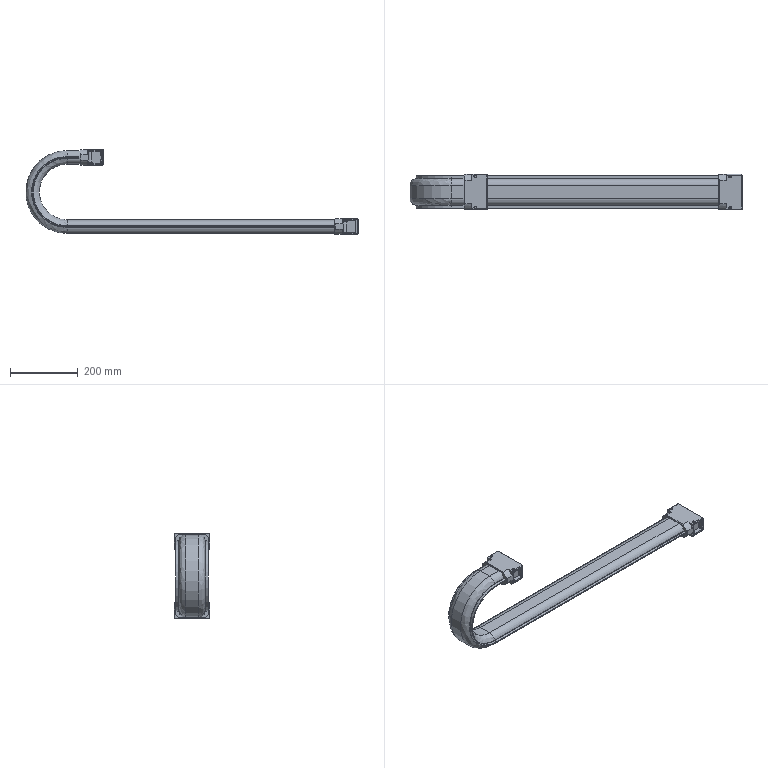Part | SolidWorks | features BaseBody 3, ICE 1 | 16 solids | 532 faces | box 978 x 104 x 250 mm | volume 1591842 mm3 | cylinder 250 | plane 214 | cone 46 | spline 22 | commonest cylinder face diameters 8 x40 5.8 x32 7.9 x32 8.9 x32 4 x24 31.505 x14